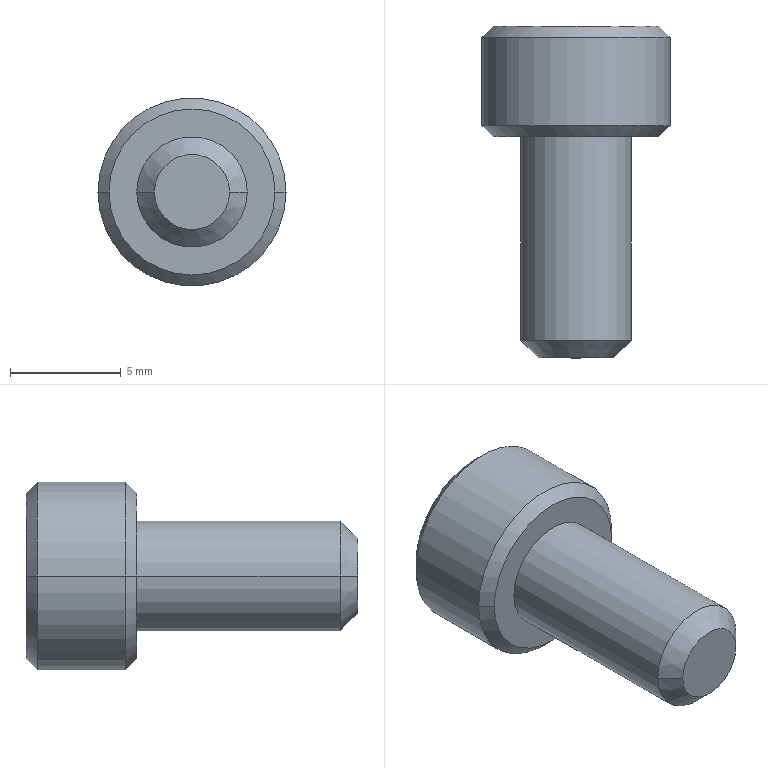Part | STEP file | BB62-M5-10L-1 | 1 solid | 27 faces | box 8.5 x 15 x 8.5 mm | volume 427.848 mm3 | plane 15 | cone 8 | cylinder 4 | commonest cylinder face diameters 5 x2 8.5 x2
STEP:
#1=CARTESIAN_POINT('',(0.,1.178,0.));
#2=VERTEX_POINT('',#1);
#3=CARTESIAN_POINT('',(2.29,2.5,0.));
#4=VERTEX_POINT('',#3);
#5=CARTESIAN_POINT('',(0.,1.178,0.));
#6=DIRECTION('',(0.866,0.5,0.));
#7=VECTOR('',#6,1000.);
#8=LINE('',#5,#7);
#9=EDGE_CURVE('',#2,#4,#8,.T.);
#10=ORIENTED_EDGE('',*,*,#9,.F.);
#11=CARTESIAN_POINT('',(-2.29,2.5,0.));
#12=VERTEX_POINT('',#11);
#13=CARTESIAN_POINT('',(0.,1.178,0.));
#14=DIRECTION('',(-0.866,0.5,0.));
#15=VECTOR('',#14,1000.);
#16=LINE('',#13,#15);
#17=EDGE_CURVE('',#2,#12,#16,.T.);
#18=ORIENTED_EDGE('',*,*,#17,.T.);
#19=CARTESIAN_POINT('',(-1.983,2.5,1.145));
#20=VERTEX_POINT('',#19);
#21=CARTESIAN_POINT('',(0.,2.5,0.));
#22=DIRECTION('',(0.,-1.,0.));
#23=DIRECTION('',(-1.,0.,0.));
#24=AXIS2_PLACEMENT_3D('',#21,#22,#23);
#25=CIRCLE('',#24,2.29);
#26=EDGE_CURVE('',#20,#12,#25,.T.);
#27=ORIENTED_EDGE('',*,*,#26,.F.);
#28=CARTESIAN_POINT('',(0.,2.5,2.29));
#29=VERTEX_POINT('',#28);
#30=CARTESIAN_POINT('',(0.,2.5,0.));
#31=DIRECTION('',(0.,-1.,0.));
#32=DIRECTION('',(-1.,0.,0.));
#33=AXIS2_PLACEMENT_3D('',#30,#31,#32);
#34=CIRCLE('',#33,2.29);
#35=EDGE_CURVE('',#29,#20,#34,.T.);
#36=ORIENTED_EDGE('',*,*,#35,.F.);
#37=CARTESIAN_POINT('',(1.983,2.5,1.145));
#38=VERTEX_POINT('',#37);
#39=CARTESIAN_POINT('',(0.,2.5,0.));
#40=DIRECTION('',(0.,-1.,0.));
#41=DIRECTION('',(-1.,0.,0.));
#42=AXIS2_PLACEMENT_3D('',#39,#40,#41);
#43=CIRCLE('',#42,2.29);
#44=EDGE_CURVE('',#38,#29,#43,.T.);
#45=ORIENTED_EDGE('',*,*,#44,.F.);
#46=CARTESIAN_POINT('',(0.,2.5,0.));
#47=DIRECTION('',(0.,-1.,0.));
#48=DIRECTION('',(-1.,0.,0.));
#49=AXIS2_PLACEMENT_3D('',#46,#47,#48);
#50=CIRCLE('',#49,2.29);
#51=EDGE_CURVE('',#4,#38,#50,.T.);
#52=ORIENTED_EDGE('',*,*,#51,.F.);
#53=EDGE_LOOP('',(#10,#18,#27,#36,#45,#52));
#54=FACE_OUTER_BOUND('',#53,.T.);
#55=CARTESIAN_POINT('',(0.,1001.178,0.));
#56=DIRECTION('',(0.,1.,0.));
#57=DIRECTION('',(1.,0.,0.));
#58=AXIS2_PLACEMENT_3D('',#55,#56,#57);
#59=CONICAL_SURFACE('',#58,1732.051,1.047);
#60=ADVANCED_FACE('',(#54),#59,.F.);
#61=CARTESIAN_POINT('',(1.7,-10.,0.));
#62=VERTEX_POINT('',#61);
#63=CARTESIAN_POINT('',(-1.7,-10.,0.));
#64=VERTEX_POINT('',#63);
#65=CARTESIAN_POINT('',(0.,-10.,0.));
#66=DIRECTION('',(0.,1.,0.));
#67=DIRECTION('',(1.,0.,0.));
#68=AXIS2_PLACEMENT_3D('',#65,#66,#67);
#69=CIRCLE('',#68,1.7);
#70=EDGE_CURVE('',#62,#64,#69,.T.);
#71=ORIENTED_EDGE('',*,*,#70,.T.);
#72=CARTESIAN_POINT('',(-2.5,-9.2,0.));
#73=VERTEX_POINT('',#72);
#74=CARTESIAN_POINT('',(-1.7,-10.,0.));
#75=DIRECTION('',(-0.7071,0.7071,0.));
#76=VECTOR('',#75,1000.);
#77=LINE('',#74,#76);
#78=EDGE_CURVE('',#64,#73,#77,.T.);
#79=ORIENTED_EDGE('',*,*,#78,.T.);
#80=CARTESIAN_POINT('',(2.5,-9.2,0.));
#81=VERTEX_POINT('',#80);
#82=CARTESIAN_POINT('',(0.,-9.2,0.));
#83=DIRECTION('',(0.,-1.,0.));
#84=DIRECTION('',(-1.,0.,0.));
#85=AXIS2_PLACEMENT_3D('',#82,#83,#84);
#86=CIRCLE('',#85,2.5);
#87=EDGE_CURVE('',#73,#81,#86,.T.);
#88=ORIENTED_EDGE('',*,*,#87,.T.);
#89=CARTESIAN_POINT('',(1.7,-10.,0.));
#90=DIRECTION('',(0.7071,0.7071,0.));
#91=VECTOR('',#90,1000.);
#92=LINE('',#89,#91);
#93=EDGE_CURVE('',#62,#81,#92,.T.);
#94=ORIENTED_EDGE('',*,*,#93,.F.);
#95=EDGE_LOOP('',(#71,#79,#88,#94));
#96=FACE_OUTER_BOUND('',#95,.T.);
#97=CARTESIAN_POINT('',(0.,-10.,0.));
#98=DIRECTION('',(0.,1.,0.));
#99=DIRECTION('',(1.,0.,0.));
#100=AXIS2_PLACEMENT_3D('',#97,#98,#99);
#101=CONICAL_SURFACE('',#100,1.7,0.7854);
#102=ADVANCED_FACE('',(#96),#101,.T.);
#103=ORIENTED_EDGE('',*,*,#87,.F.);
#104=CARTESIAN_POINT('',(-2.5,0.,0.));
#105=VERTEX_POINT('',#104);
#106=CARTESIAN_POINT('',(-2.5,-9.2,0.));
#107=DIRECTION('',(0.,1.,0.));
#108=VECTOR('',#107,1000.);
#109=LINE('',#106,#108);
#110=EDGE_CURVE('',#73,#105,#109,.T.);
#111=ORIENTED_EDGE('',*,*,#110,.T.);
#112=CARTESIAN_POINT('',(2.5,0.,0.));
#113=VERTEX_POINT('',#112);
#114=CARTESIAN_POINT('',(0.,0.,0.));
#115=DIRECTION('',(0.,-1.,0.));
#116=DIRECTION('',(-1.,0.,0.));
#117=AXIS2_PLACEMENT_3D('',#114,#115,#116);
#118=CIRCLE('',#117,2.5);
#119=EDGE_CURVE('',#105,#113,#118,.T.);
#120=ORIENTED_EDGE('',*,*,#119,.T.);
#121=CARTESIAN_POINT('',(2.5,-9.2,0.));
#122=DIRECTION('',(0.,1.,0.));
#123=VECTOR('',#122,1000.);
#124=LINE('',#121,#123);
#125=EDGE_CURVE('',#81,#113,#124,.T.);
#126=ORIENTED_EDGE('',*,*,#125,.F.);
#127=EDGE_LOOP('',(#103,#111,#120,#126));
#128=FACE_OUTER_BOUND('',#127,.T.);
#129=CARTESIAN_POINT('',(0.,-9.2,0.));
#130=DIRECTION('',(0.,1.,0.));
#131=DIRECTION('',(1.,0.,0.));
#132=AXIS2_PLACEMENT_3D('',#129,#130,#131);
#133=CYLINDRICAL_SURFACE('',#132,2.5);
#134=ADVANCED_FACE('',(#128),#133,.T.);
#135=CARTESIAN_POINT('',(-3.75,5.,0.));
#136=VERTEX_POINT('',#135);
#137=CARTESIAN_POINT('',(3.75,5.,0.));
#138=VERTEX_POINT('',#137);
#139=CARTESIAN_POINT('',(0.,5.,0.));
#140=DIRECTION('',(0.,-1.,0.));
#141=DIRECTION('',(-1.,0.,0.));
#142=AXIS2_PLACEMENT_3D('',#139,#140,#141);
#143=CIRCLE('',#142,3.75);
#144=EDGE_CURVE('',#136,#138,#143,.T.);
#145=ORIENTED_EDGE('',*,*,#144,.T.);
#146=CARTESIAN_POINT('',(4.25,4.5,0.));
#147=VERTEX_POINT('',#146);
#148=CARTESIAN_POINT('',(4.25,4.5,0.));
#149=DIRECTION('',(0.7071,-0.7071,0.));
#150=VECTOR('',#149,1000.);
#151=LINE('',#148,#150);
#152=EDGE_CURVE('',#138,#147,#151,.T.);
#153=ORIENTED_EDGE('',*,*,#152,.T.);
#154=CARTESIAN_POINT('',(-4.25,4.5,0.));
#155=VERTEX_POINT('',#154);
#156=CARTESIAN_POINT('',(0.,4.5,0.));
#157=DIRECTION('',(0.,-1.,0.));
#158=DIRECTION('',(-1.,0.,0.));
#159=AXIS2_PLACEMENT_3D('',#156,#157,#158);
#160=CIRCLE('',#159,4.25);
#161=EDGE_CURVE('',#155,#147,#160,.T.);
#162=ORIENTED_EDGE('',*,*,#161,.F.);
#163=CARTESIAN_POINT('',(-4.25,4.5,0.));
#164=DIRECTION('',(-0.7071,-0.7071,0.));
#165=VECTOR('',#164,1000.);
#166=LINE('',#163,#165);
#167=EDGE_CURVE('',#136,#155,#166,.T.);
#168=ORIENTED_EDGE('',*,*,#167,.F.);
#169=EDGE_LOOP('',(#145,#153,#162,#168));
#170=FACE_OUTER_BOUND('',#169,.T.);
#171=CARTESIAN_POINT('',(0.,4.5,0.));
#172=DIRECTION('',(0.,-1.,0.));
#173=DIRECTION('',(-1.,0.,0.));
#174=AXIS2_PLACEMENT_3D('',#171,#172,#173);
#175=CONICAL_SURFACE('',#174,4.25,0.7854);
#176=ADVANCED_FACE('',(#170),#175,.T.);
#177=ORIENTED_EDGE('',*,*,#161,.T.);
#178=CARTESIAN_POINT('',(4.25,0.5,0.));
#179=VERTEX_POINT('',#178);
#180=CARTESIAN_POINT('',(4.25,1.62,0.));
#181=DIRECTION('',(0.,-1.,0.));
#182=VECTOR('',#181,1000.);
#183=LINE('',#180,#182);
#184=EDGE_CURVE('',#147,#179,#183,.T.);
#185=ORIENTED_EDGE('',*,*,#184,.T.);
#186=CARTESIAN_POINT('',(-4.25,0.5,0.));
#187=VERTEX_POINT('',#186);
#188=CARTESIAN_POINT('',(0.,0.5,0.));
#189=DIRECTION('',(0.,-1.,0.));
#190=DIRECTION('',(-1.,0.,0.));
#191=AXIS2_PLACEMENT_3D('',#188,#189,#190);
#192=CIRCLE('',#191,4.25);
#193=EDGE_CURVE('',#187,#179,#192,.T.);
#194=ORIENTED_EDGE('',*,*,#193,.F.);
#195=CARTESIAN_POINT('',(-4.25,1.62,0.));
#196=DIRECTION('',(0.,-1.,0.));
#197=VECTOR('',#196,1000.);
#198=LINE('',#195,#197);
#199=EDGE_CURVE('',#155,#187,#198,.T.);
#200=ORIENTED_EDGE('',*,*,#199,.F.);
#201=EDGE_LOOP('',(#177,#185,#194,#200));
#202=FACE_OUTER_BOUND('',#201,.T.);
#203=CARTESIAN_POINT('',(0.,1.62,0.));
#204=DIRECTION('',(0.,-1.,0.));
#205=DIRECTION('',(-1.,0.,0.));
#206=AXIS2_PLACEMENT_3D('',#203,#204,#205);
#207=CYLINDRICAL_SURFACE('',#206,4.25);
#208=ADVANCED_FACE('',(#202),#207,.T.);
#209=CARTESIAN_POINT('',(-3.75,0.,0.));
#210=VERTEX_POINT('',#209);
#211=CARTESIAN_POINT('',(3.75,0.,0.));
#212=VERTEX_POINT('',#211);
#213=CARTESIAN_POINT('',(0.,0.,0.));
#214=DIRECTION('',(0.,-1.,0.));
#215=DIRECTION('',(-1.,0.,0.));
#216=AXIS2_PLACEMENT_3D('',#213,#214,#215);
#217=CIRCLE('',#216,3.75);
#218=EDGE_CURVE('',#210,#212,#217,.T.);
#219=ORIENTED_EDGE('',*,*,#218,.F.);
#220=CARTESIAN_POINT('',(-3.75,0.,0.));
#221=DIRECTION('',(-0.7071,0.7071,0.));
#222=VECTOR('',#221,1000.);
#223=LINE('',#220,#222);
#224=EDGE_CURVE('',#210,#187,#223,.T.);
#225=ORIENTED_EDGE('',*,*,#224,.T.);
#226=ORIENTED_EDGE('',*,*,#193,.T.);
#227=CARTESIAN_POINT('',(3.75,0.,0.));
#228=DIRECTION('',(0.7071,0.7071,0.));
#229=VECTOR('',#228,1000.);
#230=LINE('',#227,#229);
#231=EDGE_CURVE('',#212,#179,#230,.T.);
#232=ORIENTED_EDGE('',*,*,#231,.F.);
#233=EDGE_LOOP('',(#219,#225,#226,#232));
#234=FACE_OUTER_BOUND('',#233,.T.);
#235=CARTESIAN_POINT('',(0.,0.,0.));
#236=DIRECTION('',(0.,1.,0.));
#237=DIRECTION('',(1.,0.,0.));
#238=AXIS2_PLACEMENT_3D('',#235,#236,#237);
#239=CONICAL_SURFACE('',#238,3.75,0.7854);
#240=ADVANCED_FACE('',(#234),#239,.T.);
#241=ORIENTED_EDGE('',*,*,#144,.F.);
#242=CARTESIAN_POINT('',(0.,5.,0.));
#243=DIRECTION('',(0.,-1.,0.));
#244=DIRECTION('',(-1.,0.,0.));
#245=AXIS2_PLACEMENT_3D('',#242,#243,#244);
#246=CIRCLE('',#245,3.75);
#247=EDGE_CURVE('',#138,#136,#246,.T.);
#248=ORIENTED_EDGE('',*,*,#247,.F.);
#249=EDGE_LOOP('',(#241,#248));
#250=FACE_OUTER_BOUND('',#249,.T.);
#251=CARTESIAN_POINT('',(0.,5.,-2.29));
#252=VERTEX_POINT('',#251);
#253=CARTESIAN_POINT('',(-1.983,5.,-1.145));
#254=VERTEX_POINT('',#253);
#255=CARTESIAN_POINT('',(0.,5.,-2.29));
#256=DIRECTION('',(-0.866,0.,0.5));
#257=VECTOR('',#256,1000.);
#258=LINE('',#255,#257);
#259=EDGE_CURVE('',#252,#254,#258,.T.);
#260=ORIENTED_EDGE('',*,*,#259,.F.);
#261=CARTESIAN_POINT('',(1.983,5.,-1.145));
#262=VERTEX_POINT('',#261);
#263=CARTESIAN_POINT('',(1.983,5.,-1.145));
#264=DIRECTION('',(-0.866,0.,-0.5));
#265=VECTOR('',#264,1000.);
#266=LINE('',#263,#265);
#267=EDGE_CURVE('',#262,#252,#266,.T.);
#268=ORIENTED_EDGE('',*,*,#267,.F.);
#269=CARTESIAN_POINT('',(1.983,5.,1.145));
#270=VERTEX_POINT('',#269);
#271=CARTESIAN_POINT('',(1.983,5.,1.145));
#272=DIRECTION('',(0.,0.,-1.));
#273=VECTOR('',#272,1000.);
#274=LINE('',#271,#273);
#275=EDGE_CURVE('',#270,#262,#274,.T.);
#276=ORIENTED_EDGE('',*,*,#275,.F.);
#277=CARTESIAN_POINT('',(0.,5.,2.29));
#278=VERTEX_POINT('',#277);
#279=CARTESIAN_POINT('',(0.,5.,2.29));
#280=DIRECTION('',(0.866,0.,-0.5));
#281=VECTOR('',#280,1000.);
#282=LINE('',#279,#281);
#283=EDGE_CURVE('',#278,#270,#282,.T.);
#284=ORIENTED_EDGE('',*,*,#283,.F.);
#285=CARTESIAN_POINT('',(-1.983,5.,1.145));
#286=VERTEX_POINT('',#285);
#287=CARTESIAN_POINT('',(-1.983,5.,1.145));
#288=DIRECTION('',(0.866,0.,0.5));
#289=VECTOR('',#288,1000.);
#290=LINE('',#287,#289);
#291=EDGE_CURVE('',#286,#278,#290,.T.);
#292=ORIENTED_EDGE('',*,*,#291,.F.);
#293=CARTESIAN_POINT('',(-1.983,5.,-1.145));
#294=DIRECTION('',(0.,0.,1.));
#295=VECTOR('',#294,1000.);
#296=LINE('',#293,#295);
#297=EDGE_CURVE('',#254,#286,#296,.T.);
#298=ORIENTED_EDGE('',*,*,#297,.F.);
#299=EDGE_LOOP('',(#260,#268,#276,#284,#292,#298));
#300=FACE_BOUND('',#299,.T.);
#301=CARTESIAN_POINT('',(3.75,5.,0.));
#302=DIRECTION('',(0.,1.,0.));
#303=DIRECTION('',(1.,0.,0.));
#304=AXIS2_PLACEMENT_3D('',#301,#302,#303);
#305=PLANE('',#304);
#306=ADVANCED_FACE('',(#250,#300),#305,.T.);
#307=CARTESIAN_POINT('',(0.,0.,0.));
#308=DIRECTION('',(0.,-1.,0.));
#309=DIRECTION('',(-1.,0.,0.));
#310=AXIS2_PLACEMENT_3D('',#307,#308,#309);
#311=CIRCLE('',#310,2.5);
#312=EDGE_CURVE('',#113,#105,#311,.T.);
#313=ORIENTED_EDGE('',*,*,#312,.F.);
#314=ORIENTED_EDGE('',*,*,#119,.F.);
#315=EDGE_LOOP('',(#313,#314));
#316=FACE_BOUND('',#315,.T.);
#317=CARTESIAN_POINT('',(0.,0.,0.));
#318=DIRECTION('',(0.,-1.,0.));
#319=DIRECTION('',(-1.,0.,0.));
#320=AXIS2_PLACEMENT_3D('',#317,#318,#319);
#321=CIRCLE('',#320,3.75);
#322=EDGE_CURVE('',#212,#210,#321,.T.);
#323=ORIENTED_EDGE('',*,*,#322,.T.);
#324=ORIENTED_EDGE('',*,*,#218,.T.);
#325=EDGE_LOOP('',(#323,#324));
#326=FACE_OUTER_BOUND('',#325,.T.);
#327=CARTESIAN_POINT('',(0.,0.,0.));
#328=DIRECTION('',(0.,-1.,0.));
#329=DIRECTION('',(-1.,0.,0.));
#330=AXIS2_PLACEMENT_3D('',#327,#328,#329);
#331=PLANE('',#330);
#332=ADVANCED_FACE('',(#316,#326),#331,.T.);
#333=ORIENTED_EDGE('',*,*,#224,.F.);
#334=ORIENTED_EDGE('',*,*,#322,.F.);
#335=ORIENTED_EDGE('',*,*,#231,.T.);
#336=CARTESIAN_POINT('',(0.,0.5,0.));
#337=DIRECTION('',(0.,-1.,0.));
#338=DIRECTION('',(-1.,0.,0.));
#339=AXIS2_PLACEMENT_3D('',#336,#337,#338);
#340=CIRCLE('',#339,4.25);
#341=EDGE_CURVE('',#179,#187,#340,.T.);
#342=ORIENTED_EDGE('',*,*,#341,.T.);
#343=EDGE_LOOP('',(#333,#334,#335,#342));
#344=FACE_OUTER_BOUND('',#343,.T.);
#345=CARTESIAN_POINT('',(0.,0.,0.));
#346=DIRECTION('',(0.,1.,0.));
#347=DIRECTION('',(1.,0.,0.));
#348=AXIS2_PLACEMENT_3D('',#345,#346,#347);
#349=CONICAL_SURFACE('',#348,3.75,0.7854);
#350=ADVANCED_FACE('',(#344),#349,.T.);
#351=ORIENTED_EDGE('',*,*,#184,.F.);
#352=CARTESIAN_POINT('',(0.,4.5,0.));
#353=DIRECTION('',(0.,-1.,0.));
#354=DIRECTION('',(-1.,0.,0.));
#355=AXIS2_PLACEMENT_3D('',#352,#353,#354);
#356=CIRCLE('',#355,4.25);
#357=EDGE_CURVE('',#147,#155,#356,.T.);
#358=ORIENTED_EDGE('',*,*,#357,.T.);
#359=ORIENTED_EDGE('',*,*,#199,.T.);
#360=ORIENTED_EDGE('',*,*,#341,.F.);
#361=EDGE_LOOP('',(#351,#358,#359,#360));
#362=FACE_OUTER_BOUND('',#361,.T.);
#363=CARTESIAN_POINT('',(0.,1.62,0.));
#364=DIRECTION('',(0.,-1.,0.));
#365=DIRECTION('',(-1.,0.,0.));
#366=AXIS2_PLACEMENT_3D('',#363,#364,#365);
#367=CYLINDRICAL_SURFACE('',#366,4.25);
#368=ADVANCED_FACE('',(#362),#367,.T.);
#369=ORIENTED_EDGE('',*,*,#152,.F.);
#370=ORIENTED_EDGE('',*,*,#247,.T.);
#371=ORIENTED_EDGE('',*,*,#167,.T.);
#372=ORIENTED_EDGE('',*,*,#357,.F.);
#373=EDGE_LOOP('',(#369,#370,#371,#372));
#374=FACE_OUTER_BOUND('',#373,.T.);
#375=CARTESIAN_POINT('',(0.,4.5,0.));
#376=DIRECTION('',(0.,-1.,0.));
#377=DIRECTION('',(-1.,0.,0.));
#378=AXIS2_PLACEMENT_3D('',#375,#376,#377);
#379=CONICAL_SURFACE('',#378,4.25,0.7854);
#380=ADVANCED_FACE('',(#374),#379,.T.);
#381=ORIENTED_EDGE('',*,*,#110,.F.);
#382=CARTESIAN_POINT('',(0.,-9.2,0.));
#383=DIRECTION('',(0.,-1.,0.));
#384=DIRECTION('',(-1.,0.,0.));
#385=AXIS2_PLACEMENT_3D('',#382,#383,#384);
#386=CIRCLE('',#385,2.5);
#387=EDGE_CURVE('',#81,#73,#386,.T.);
#388=ORIENTED_EDGE('',*,*,#387,.F.);
#389=ORIENTED_EDGE('',*,*,#125,.T.);
#390=ORIENTED_EDGE('',*,*,#312,.T.);
#391=EDGE_LOOP('',(#381,#388,#389,#390));
#392=FACE_OUTER_BOUND('',#391,.T.);
#393=CARTESIAN_POINT('',(0.,-9.2,0.));
#394=DIRECTION('',(0.,1.,0.));
#395=DIRECTION('',(1.,0.,0.));
#396=AXIS2_PLACEMENT_3D('',#393,#394,#395);
#397=CYLINDRICAL_SURFACE('',#396,2.5);
#398=ADVANCED_FACE('',(#392),#397,.T.);
#399=ORIENTED_EDGE('',*,*,#70,.F.);
#400=CARTESIAN_POINT('',(0.,-10.,0.));
#401=DIRECTION('',(0.,1.,0.));
#402=DIRECTION('',(1.,0.,0.));
#403=AXIS2_PLACEMENT_3D('',#400,#401,#402);
#404=CIRCLE('',#403,1.7);
#405=EDGE_CURVE('',#64,#62,#404,.T.);
#406=ORIENTED_EDGE('',*,*,#405,.F.);
#407=EDGE_LOOP('',(#399,#406));
#408=FACE_OUTER_BOUND('',#407,.T.);
#409=CARTESIAN_POINT('',(0.,-10.,0.));
#410=DIRECTION('',(0.,-1.,0.));
#411=DIRECTION('',(-1.,0.,0.));
#412=AXIS2_PLACEMENT_3D('',#409,#410,#411);
#413=PLANE('',#412);
#414=ADVANCED_FACE('',(#408),#413,.T.);
#415=ORIENTED_EDGE('',*,*,#78,.F.);
#416=ORIENTED_EDGE('',*,*,#405,.T.);
#417=ORIENTED_EDGE('',*,*,#93,.T.);
#418=ORIENTED_EDGE('',*,*,#387,.T.);
#419=EDGE_LOOP('',(#415,#416,#417,#418));
#420=FACE_OUTER_BOUND('',#419,.T.);
#421=CARTESIAN_POINT('',(0.,-10.,0.));
#422=DIRECTION('',(0.,1.,0.));
#423=DIRECTION('',(1.,0.,0.));
#424=AXIS2_PLACEMENT_3D('',#421,#422,#423);
#425=CONICAL_SURFACE('',#424,1.7,0.7854);
#426=ADVANCED_FACE('',(#420),#425,.T.);
#427=CARTESIAN_POINT('',(1.983,2.5,-1.145));
#428=VERTEX_POINT('',#427);
#429=CARTESIAN_POINT('',(0.,2.5,-2.29));
#430=VERTEX_POINT('',#429);
#431=CARTESIAN_POINT('',(1.983,2.5,-1.145));
#432=DIRECTION('',(-0.866,0.,-0.5));
#433=VECTOR('',#432,1000.);
#434=LINE('',#431,#433);
#435=EDGE_CURVE('',#428,#430,#434,.T.);
#436=ORIENTED_EDGE('',*,*,#435,.F.);
#437=CARTESIAN_POINT('',(1.983,5.,-1.145));
#438=DIRECTION('',(0.,-1.,0.));
#439=VECTOR('',#438,1000.);
#440=LINE('',#437,#439);
#441=EDGE_CURVE('',#262,#428,#440,.T.);
#442=ORIENTED_EDGE('',*,*,#441,.F.);
#443=ORIENTED_EDGE('',*,*,#267,.T.);
#444=CARTESIAN_POINT('',(0.,5.,-2.29));
#445=DIRECTION('',(0.,-1.,0.));
#446=VECTOR('',#445,1000.);
#447=LINE('',#444,#446);
#448=EDGE_CURVE('',#252,#430,#447,.T.);
#449=ORIENTED_EDGE('',*,*,#448,.T.);
#450=EDGE_LOOP('',(#436,#442,#443,#449));
#451=FACE_OUTER_BOUND('',#450,.T.);
#452=CARTESIAN_POINT('',(1.983,5.,-1.145));
#453=DIRECTION('',(-0.5,0.,0.866));
#454=DIRECTION('',(0.866,0.,0.5));
#455=AXIS2_PLACEMENT_3D('',#452,#453,#454);
#456=PLANE('',#455);
#457=ADVANCED_FACE('',(#451),#456,.T.);
#458=CARTESIAN_POINT('',(-1.983,2.5,-1.145));
#459=VERTEX_POINT('',#458);
#460=CARTESIAN_POINT('',(0.,2.5,-2.29));
#461=DIRECTION('',(-0.866,0.,0.5));
#462=VECTOR('',#461,1000.);
#463=LINE('',#460,#462);
#464=EDGE_CURVE('',#430,#459,#463,.T.);
#465=ORIENTED_EDGE('',*,*,#464,.F.);
#466=ORIENTED_EDGE('',*,*,#448,.F.);
#467=ORIENTED_EDGE('',*,*,#259,.T.);
#468=CARTESIAN_POINT('',(-1.983,5.,-1.145));
#469=DIRECTION('',(0.,-1.,0.));
#470=VECTOR('',#469,1000.);
#471=LINE('',#468,#470);
#472=EDGE_CURVE('',#254,#459,#471,.T.);
#473=ORIENTED_EDGE('',*,*,#472,.T.);
#474=EDGE_LOOP('',(#465,#466,#467,#473));
#475=FACE_OUTER_BOUND('',#474,.T.);
#476=CARTESIAN_POINT('',(0.,5.,-2.29));
#477=DIRECTION('',(0.5,0.,0.866));
#478=DIRECTION('',(0.866,0.,-0.5));
#479=AXIS2_PLACEMENT_3D('',#476,#477,#478);
#480=PLANE('',#479);
#481=ADVANCED_FACE('',(#475),#480,.T.);
#482=CARTESIAN_POINT('',(-1.983,2.5,-1.145));
#483=DIRECTION('',(0.,0.,1.));
#484=VECTOR('',#483,1000.);
#485=LINE('',#482,#484);
#486=EDGE_CURVE('',#459,#20,#485,.T.);
#487=ORIENTED_EDGE('',*,*,#486,.F.);
#488=ORIENTED_EDGE('',*,*,#472,.F.);
#489=ORIENTED_EDGE('',*,*,#297,.T.);
#490=CARTESIAN_POINT('',(-1.983,5.,1.145));
#491=DIRECTION('',(0.,-1.,0.));
#492=VECTOR('',#491,1000.);
#493=LINE('',#490,#492);
#494=EDGE_CURVE('',#286,#20,#493,.T.);
#495=ORIENTED_EDGE('',*,*,#494,.T.);
#496=EDGE_LOOP('',(#487,#488,#489,#495));
#497=FACE_OUTER_BOUND('',#496,.T.);
#498=CARTESIAN_POINT('',(-1.983,5.,-1.145));
#499=DIRECTION('',(1.,0.,0.));
#500=DIRECTION('',(0.,0.,-1.));
#501=AXIS2_PLACEMENT_3D('',#498,#499,#500);
#502=PLANE('',#501);
#503=ADVANCED_FACE('',(#497),#502,.T.);
#504=CARTESIAN_POINT('',(-1.983,2.5,1.145));
#505=DIRECTION('',(0.866,0.,0.5));
#506=VECTOR('',#505,1000.);
#507=LINE('',#504,#506);
#508=EDGE_CURVE('',#20,#29,#507,.T.);
#509=ORIENTED_EDGE('',*,*,#508,.F.);
#510=ORIENTED_EDGE('',*,*,#494,.F.);
#511=ORIENTED_EDGE('',*,*,#291,.T.);
#512=CARTESIAN_POINT('',(0.,5.,2.29));
#513=DIRECTION('',(0.,-1.,0.));
#514=VECTOR('',#513,1000.);
#515=LINE('',#512,#514);
#516=EDGE_CURVE('',#278,#29,#515,.T.);
#517=ORIENTED_EDGE('',*,*,#516,.T.);
#518=EDGE_LOOP('',(#509,#510,#511,#517));
#519=FACE_OUTER_BOUND('',#518,.T.);
#520=CARTESIAN_POINT('',(-1.983,5.,1.145));
#521=DIRECTION('',(0.5,0.,-0.866));
#522=DIRECTION('',(-0.866,0.,-0.5));
#523=AXIS2_PLACEMENT_3D('',#520,#521,#522);
#524=PLANE('',#523);
#525=ADVANCED_FACE('',(#519),#524,.T.);
#526=CARTESIAN_POINT('',(0.,2.5,2.29));
#527=DIRECTION('',(0.866,0.,-0.5));
#528=VECTOR('',#527,1000.);
#529=LINE('',#526,#528);
#530=EDGE_CURVE('',#29,#38,#529,.T.);
#531=ORIENTED_EDGE('',*,*,#530,.F.);
#532=ORIENTED_EDGE('',*,*,#516,.F.);
#533=ORIENTED_EDGE('',*,*,#283,.T.);
#534=CARTESIAN_POINT('',(1.983,5.,1.145));
#535=DIRECTION('',(0.,-1.,0.));
#536=VECTOR('',#535,1000.);
#537=LINE('',#534,#536);
#538=EDGE_CURVE('',#270,#38,#537,.T.);
#539=ORIENTED_EDGE('',*,*,#538,.T.);
#540=EDGE_LOOP('',(#531,#532,#533,#539));
#541=FACE_OUTER_BOUND('',#540,.T.);
#542=CARTESIAN_POINT('',(0.,5.,2.29));
#543=DIRECTION('',(-0.5,0.,-0.866));
#544=DIRECTION('',(-0.866,0.,0.5));
#545=AXIS2_PLACEMENT_3D('',#542,#543,#544);
#546=PLANE('',#545);
#547=ADVANCED_FACE('',(#541),#546,.T.);
#548=CARTESIAN_POINT('',(1.983,2.5,1.145));
#549=DIRECTION('',(0.,0.,-1.));
#550=VECTOR('',#549,1000.);
#551=LINE('',#548,#550);
#552=EDGE_CURVE('',#38,#428,#551,.T.);
#553=ORIENTED_EDGE('',*,*,#552,.F.);
#554=ORIENTED_EDGE('',*,*,#538,.F.);
#555=ORIENTED_EDGE('',*,*,#275,.T.);
#556=ORIENTED_EDGE('',*,*,#441,.T.);
#557=EDGE_LOOP('',(#553,#554,#555,#556));
#558=FACE_OUTER_BOUND('',#557,.T.);
#559=CARTESIAN_POINT('',(1.983,5.,1.145));
#560=DIRECTION('',(-1.,0.,0.));
#561=DIRECTION('',(0.,0.,1.));
#562=AXIS2_PLACEMENT_3D('',#559,#560,#561);
#563=PLANE('',#562);
#564=ADVANCED_FACE('',(#558),#563,.T.);
#565=ORIENTED_EDGE('',*,*,#435,.T.);
#566=CARTESIAN_POINT('',(0.,2.5,0.));
#567=DIRECTION('',(0.,-1.,0.));
#568=DIRECTION('',(-1.,0.,0.));
#569=AXIS2_PLACEMENT_3D('',#566,#567,#568);
#570=CIRCLE('',#569,2.29);
#571=EDGE_CURVE('',#430,#428,#570,.T.);
#572=ORIENTED_EDGE('',*,*,#571,.T.);
#573=EDGE_LOOP('',(#565,#572));
#574=FACE_OUTER_BOUND('',#573,.T.);
#575=CARTESIAN_POINT('',(0.,2.5,0.));
#576=DIRECTION('',(0.,1.,0.));
#577=DIRECTION('',(1.,0.,0.));
#578=AXIS2_PLACEMENT_3D('',#575,#576,#577);
#579=PLANE('',#578);
#580=ADVANCED_FACE('',(#574),#579,.F.);
#581=ORIENTED_EDGE('',*,*,#552,.T.);
#582=CARTESIAN_POINT('',(0.,2.5,0.));
#583=DIRECTION('',(0.,-1.,0.));
#584=DIRECTION('',(-1.,0.,0.));
#585=AXIS2_PLACEMENT_3D('',#582,#583,#584);
#586=CIRCLE('',#585,2.29);
#587=EDGE_CURVE('',#428,#4,#586,.T.);
#588=ORIENTED_EDGE('',*,*,#587,.T.);
#589=ORIENTED_EDGE('',*,*,#51,.T.);
#590=EDGE_LOOP('',(#581,#588,#589));
#591=FACE_OUTER_BOUND('',#590,.T.);
#592=CARTESIAN_POINT('',(0.,2.5,0.));
#593=DIRECTION('',(0.,1.,0.));
#594=DIRECTION('',(1.,0.,0.));
#595=AXIS2_PLACEMENT_3D('',#592,#593,#594);
#596=PLANE('',#595);
#597=ADVANCED_FACE('',(#591),#596,.F.);
#598=ORIENTED_EDGE('',*,*,#530,.T.);
#599=ORIENTED_EDGE('',*,*,#44,.T.);
#600=EDGE_LOOP('',(#598,#599));
#601=FACE_OUTER_BOUND('',#600,.T.);
#602=CARTESIAN_POINT('',(0.,2.5,0.));
#603=DIRECTION('',(0.,1.,0.));
#604=DIRECTION('',(1.,0.,0.));
#605=AXIS2_PLACEMENT_3D('',#602,#603,#604);
#606=PLANE('',#605);
#607=ADVANCED_FACE('',(#601),#606,.F.);
#608=ORIENTED_EDGE('',*,*,#508,.T.);
#609=ORIENTED_EDGE('',*,*,#35,.T.);
#610=EDGE_LOOP('',(#608,#609));
#611=FACE_OUTER_BOUND('',#610,.T.);
#612=CARTESIAN_POINT('',(0.,2.5,0.));
#613=DIRECTION('',(0.,1.,0.));
#614=DIRECTION('',(1.,0.,0.));
#615=AXIS2_PLACEMENT_3D('',#612,#613,#614);
#616=PLANE('',#615);
#617=ADVANCED_FACE('',(#611),#616,.F.);
#618=ORIENTED_EDGE('',*,*,#486,.T.);
#619=ORIENTED_EDGE('',*,*,#26,.T.);
#620=CARTESIAN_POINT('',(0.,2.5,0.));
#621=DIRECTION('',(0.,-1.,0.));
#622=DIRECTION('',(-1.,0.,0.));
#623=AXIS2_PLACEMENT_3D('',#620,#621,#622);
#624=CIRCLE('',#623,2.29);
#625=EDGE_CURVE('',#12,#459,#624,.T.);
#626=ORIENTED_EDGE('',*,*,#625,.T.);
#627=EDGE_LOOP('',(#618,#619,#626));
#628=FACE_OUTER_BOUND('',#627,.T.);
#629=CARTESIAN_POINT('',(0.,2.5,0.));
#630=DIRECTION('',(0.,1.,0.));
#631=DIRECTION('',(1.,0.,0.));
#632=AXIS2_PLACEMENT_3D('',#629,#630,#631);
#633=PLANE('',#632);
#634=ADVANCED_FACE('',(#628),#633,.F.);
#635=ORIENTED_EDGE('',*,*,#464,.T.);
#636=CARTESIAN_POINT('',(0.,2.5,0.));
#637=DIRECTION('',(0.,-1.,0.));
#638=DIRECTION('',(-1.,0.,0.));
#639=AXIS2_PLACEMENT_3D('',#636,#637,#638);
#640=CIRCLE('',#639,2.29);
#641=EDGE_CURVE('',#459,#430,#640,.T.);
#642=ORIENTED_EDGE('',*,*,#641,.T.);
#643=EDGE_LOOP('',(#635,#642));
#644=FACE_OUTER_BOUND('',#643,.T.);
#645=CARTESIAN_POINT('',(0.,2.5,0.));
#646=DIRECTION('',(0.,1.,0.));
#647=DIRECTION('',(1.,0.,0.));
#648=AXIS2_PLACEMENT_3D('',#645,#646,#647);
#649=PLANE('',#648);
#650=ADVANCED_FACE('',(#644),#649,.F.);
#651=ORIENTED_EDGE('',*,*,#17,.F.);
#652=ORIENTED_EDGE('',*,*,#9,.T.);
#653=ORIENTED_EDGE('',*,*,#587,.F.);
#654=ORIENTED_EDGE('',*,*,#571,.F.);
#655=ORIENTED_EDGE('',*,*,#641,.F.);
#656=ORIENTED_EDGE('',*,*,#625,.F.);
#657=EDGE_LOOP('',(#651,#652,#653,#654,#655,#656));
#658=FACE_OUTER_BOUND('',#657,.T.);
#659=CARTESIAN_POINT('',(0.,1001.178,0.));
#660=DIRECTION('',(0.,1.,0.));
#661=DIRECTION('',(1.,0.,0.));
#662=AXIS2_PLACEMENT_3D('',#659,#660,#661);
#663=CONICAL_SURFACE('',#662,1732.051,1.047);
#664=ADVANCED_FACE('',(#658),#663,.F.);
#665=CLOSED_SHELL('',(#60,#102,#134,#176,#208,#240,#306,#332,#350,#368,#380,#398,#414,#426,#457,#481,#503,#525,#547,#564,#580,#597,#607,#617,#634,#650,#664));
#666=MANIFOLD_SOLID_BREP('',#665);
#667=CARTESIAN_POINT('',(0.,0.,0.));
#668=DIRECTION('',(0.,0.,1.));
#669=DIRECTION('',(1.,0.,0.));
#670=AXIS2_PLACEMENT_3D('',#667,#668,#669);
#671=(LENGTH_UNIT()NAMED_UNIT(*)SI_UNIT(.MILLI.,.METRE.));
#672=UNCERTAINTY_MEASURE_WITH_UNIT(LENGTH_MEASURE(0.00001),#671,'','');
#673=(NAMED_UNIT(*)PLANE_ANGLE_UNIT()SI_UNIT($,.RADIAN.));
#674=(NAMED_UNIT(*)SI_UNIT($,.STERADIAN.)SOLID_ANGLE_UNIT());
#675=(GEOMETRIC_REPRESENTATION_CONTEXT(3)GLOBAL_UNCERTAINTY_ASSIGNED_CONTEXT((#672))GLOBAL_UNIT_ASSIGNED_CONTEXT((#671,#673,#674))REPRESENTATION_CONTEXT('',''));
#676=ADVANCED_BREP_SHAPE_REPRESENTATION('',(#666,#670),#675);